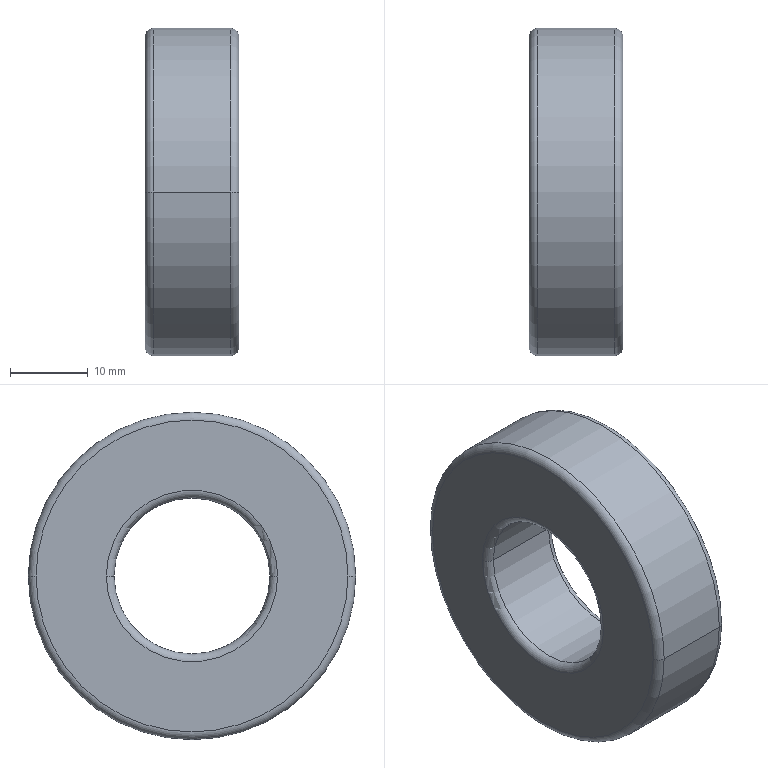Part | NX | features BREP 1 | 1 solid | 14 faces | box 12 x 42 x 42 mm | volume 12772 mm3 | torus 8 | cylinder 4 | plane 2 | commonest cylinder face diameters 20 x2 42 x2
STEP:
#1=CARTESIAN_POINT('',(12.,-20.,0.));
#2=VERTEX_POINT('',#1);
#3=CARTESIAN_POINT('',(12.,20.,0.));
#4=VERTEX_POINT('',#3);
#5=CARTESIAN_POINT('',(12.,0.,0.));
#6=DIRECTION('',(1.,0.,0.));
#7=DIRECTION('',(0.,-1.,0.));
#8=AXIS2_PLACEMENT_3D('',#5,#6,#7);
#9=CIRCLE('',#8,20.);
#10=EDGE_CURVE('',#2,#4,#9,.T.);
#11=ORIENTED_EDGE('',*,*,#10,.T.);
#12=CARTESIAN_POINT('',(12.,0.,0.));
#13=DIRECTION('',(1.,0.,0.));
#14=DIRECTION('',(0.,1.,0.));
#15=AXIS2_PLACEMENT_3D('',#12,#13,#14);
#16=CIRCLE('',#15,20.);
#17=EDGE_CURVE('',#4,#2,#16,.T.);
#18=ORIENTED_EDGE('',*,*,#17,.T.);
#19=EDGE_LOOP('',(#11,#18));
#20=FACE_BOUND('',#19,.T.);
#21=CARTESIAN_POINT('',(12.,-11.,0.));
#22=VERTEX_POINT('',#21);
#23=CARTESIAN_POINT('',(12.,11.,0.));
#24=VERTEX_POINT('',#23);
#25=CARTESIAN_POINT('',(12.,0.,0.));
#26=DIRECTION('',(-1.,0.,0.));
#27=DIRECTION('',(0.,-1.,0.));
#28=AXIS2_PLACEMENT_3D('',#25,#26,#27);
#29=CIRCLE('',#28,11.);
#30=EDGE_CURVE('',#22,#24,#29,.T.);
#31=ORIENTED_EDGE('',*,*,#30,.T.);
#32=CARTESIAN_POINT('',(12.,0.,0.));
#33=DIRECTION('',(-1.,0.,0.));
#34=DIRECTION('',(0.,1.,0.));
#35=AXIS2_PLACEMENT_3D('',#32,#33,#34);
#36=CIRCLE('',#35,11.);
#37=EDGE_CURVE('',#24,#22,#36,.T.);
#38=ORIENTED_EDGE('',*,*,#37,.T.);
#39=EDGE_LOOP('',(#31,#38));
#40=FACE_BOUND('',#39,.T.);
#41=CARTESIAN_POINT('',(12.,0.,0.));
#42=DIRECTION('',(1.,0.,0.));
#43=DIRECTION('',(0.,1.,0.));
#44=AXIS2_PLACEMENT_3D('',#41,#42,#43);
#45=PLANE('',#44);
#46=ADVANCED_FACE('',(#20,#40),#45,.T.);
#47=CARTESIAN_POINT('',(11.,21.,0.));
#48=VERTEX_POINT('',#47);
#49=CARTESIAN_POINT('',(11.,-21.,0.));
#50=VERTEX_POINT('',#49);
#51=CARTESIAN_POINT('',(11.,0.,0.));
#52=DIRECTION('',(1.,0.,0.));
#53=DIRECTION('',(0.,1.,0.));
#54=AXIS2_PLACEMENT_3D('',#51,#52,#53);
#55=CIRCLE('',#54,21.);
#56=EDGE_CURVE('',#48,#50,#55,.T.);
#57=ORIENTED_EDGE('',*,*,#56,.T.);
#58=CARTESIAN_POINT('',(11.,-20.,0.));
#59=DIRECTION('',(0.,0.,1.));
#60=DIRECTION('',(0.,-1.,0.));
#61=AXIS2_PLACEMENT_3D('',#58,#59,#60);
#62=CIRCLE('',#61,1.);
#63=EDGE_CURVE('',#50,#2,#62,.T.);
#64=ORIENTED_EDGE('',*,*,#63,.T.);
#65=ORIENTED_EDGE('',*,*,#17,.F.);
#66=CARTESIAN_POINT('',(11.,20.,0.));
#67=DIRECTION('',(0.,0.,-1.));
#68=DIRECTION('',(0.,1.,0.));
#69=AXIS2_PLACEMENT_3D('',#66,#67,#68);
#70=CIRCLE('',#69,1.);
#71=EDGE_CURVE('',#48,#4,#70,.T.);
#72=ORIENTED_EDGE('',*,*,#71,.F.);
#73=EDGE_LOOP('',(#57,#64,#65,#72));
#74=FACE_BOUND('',#73,.T.);
#75=CARTESIAN_POINT('',(11.,0.,0.));
#76=DIRECTION('',(1.,0.,0.));
#77=DIRECTION('',(0.,1.,0.));
#78=AXIS2_PLACEMENT_3D('',#75,#76,#77);
#79=TOROIDAL_SURFACE('',#78,20.,1.);
#80=ADVANCED_FACE('',(#74),#79,.T.);
#81=CARTESIAN_POINT('',(11.,0.,0.));
#82=DIRECTION('',(1.,0.,0.));
#83=DIRECTION('',(0.,-1.,0.));
#84=AXIS2_PLACEMENT_3D('',#81,#82,#83);
#85=CIRCLE('',#84,21.);
#86=EDGE_CURVE('',#50,#48,#85,.T.);
#87=ORIENTED_EDGE('',*,*,#86,.T.);
#88=ORIENTED_EDGE('',*,*,#71,.T.);
#89=ORIENTED_EDGE('',*,*,#10,.F.);
#90=ORIENTED_EDGE('',*,*,#63,.F.);
#91=EDGE_LOOP('',(#87,#88,#89,#90));
#92=FACE_BOUND('',#91,.T.);
#93=CARTESIAN_POINT('',(11.,0.,0.));
#94=DIRECTION('',(1.,0.,0.));
#95=DIRECTION('',(0.,-1.,0.));
#96=AXIS2_PLACEMENT_3D('',#93,#94,#95);
#97=TOROIDAL_SURFACE('',#96,20.,1.);
#98=ADVANCED_FACE('',(#92),#97,.T.);
#99=ORIENTED_EDGE('',*,*,#86,.F.);
#100=CARTESIAN_POINT('',(1.,-21.,0.));
#101=VERTEX_POINT('',#100);
#102=CARTESIAN_POINT('',(11.,-21.,0.));
#103=DIRECTION('',(-1.,0.,0.));
#104=VECTOR('',#103,1000.);
#105=LINE('',#102,#104);
#106=EDGE_CURVE('',#50,#101,#105,.T.);
#107=ORIENTED_EDGE('',*,*,#106,.T.);
#108=CARTESIAN_POINT('',(1.,21.,0.));
#109=VERTEX_POINT('',#108);
#110=CARTESIAN_POINT('',(1.,0.,0.));
#111=DIRECTION('',(-1.,0.,0.));
#112=DIRECTION('',(0.,1.,0.));
#113=AXIS2_PLACEMENT_3D('',#110,#111,#112);
#114=CIRCLE('',#113,21.);
#115=EDGE_CURVE('',#109,#101,#114,.T.);
#116=ORIENTED_EDGE('',*,*,#115,.F.);
#117=CARTESIAN_POINT('',(11.,21.,0.));
#118=DIRECTION('',(-1.,0.,0.));
#119=VECTOR('',#118,1000.);
#120=LINE('',#117,#119);
#121=EDGE_CURVE('',#48,#109,#120,.T.);
#122=ORIENTED_EDGE('',*,*,#121,.F.);
#123=EDGE_LOOP('',(#99,#107,#116,#122));
#124=FACE_BOUND('',#123,.T.);
#125=CARTESIAN_POINT('',(6.,0.,0.));
#126=DIRECTION('',(1.,0.,0.));
#127=DIRECTION('',(0.,1.,0.));
#128=AXIS2_PLACEMENT_3D('',#125,#126,#127);
#129=CYLINDRICAL_SURFACE('',#128,21.);
#130=ADVANCED_FACE('',(#124),#129,.T.);
#131=ORIENTED_EDGE('',*,*,#56,.F.);
#132=ORIENTED_EDGE('',*,*,#121,.T.);
#133=CARTESIAN_POINT('',(1.,0.,0.));
#134=DIRECTION('',(-1.,0.,0.));
#135=DIRECTION('',(0.,-1.,0.));
#136=AXIS2_PLACEMENT_3D('',#133,#134,#135);
#137=CIRCLE('',#136,21.);
#138=EDGE_CURVE('',#101,#109,#137,.T.);
#139=ORIENTED_EDGE('',*,*,#138,.F.);
#140=ORIENTED_EDGE('',*,*,#106,.F.);
#141=EDGE_LOOP('',(#131,#132,#139,#140));
#142=FACE_BOUND('',#141,.T.);
#143=CARTESIAN_POINT('',(6.,0.,0.));
#144=DIRECTION('',(1.,0.,0.));
#145=DIRECTION('',(0.,1.,0.));
#146=AXIS2_PLACEMENT_3D('',#143,#144,#145);
#147=CYLINDRICAL_SURFACE('',#146,21.);
#148=ADVANCED_FACE('',(#142),#147,.T.);
#149=CARTESIAN_POINT('',(0.,-20.,0.));
#150=VERTEX_POINT('',#149);
#151=CARTESIAN_POINT('',(0.,20.,0.));
#152=VERTEX_POINT('',#151);
#153=CARTESIAN_POINT('',(0.,0.,0.));
#154=DIRECTION('',(-1.,0.,0.));
#155=DIRECTION('',(0.,-1.,0.));
#156=AXIS2_PLACEMENT_3D('',#153,#154,#155);
#157=CIRCLE('',#156,20.);
#158=EDGE_CURVE('',#150,#152,#157,.T.);
#159=ORIENTED_EDGE('',*,*,#158,.F.);
#160=CARTESIAN_POINT('',(1.,-20.,0.));
#161=DIRECTION('',(0.,0.,1.));
#162=DIRECTION('',(-1.,0.,0.));
#163=AXIS2_PLACEMENT_3D('',#160,#161,#162);
#164=CIRCLE('',#163,1.);
#165=EDGE_CURVE('',#150,#101,#164,.T.);
#166=ORIENTED_EDGE('',*,*,#165,.T.);
#167=ORIENTED_EDGE('',*,*,#138,.T.);
#168=CARTESIAN_POINT('',(1.,20.,0.));
#169=DIRECTION('',(0.,0.,-1.));
#170=DIRECTION('',(-1.,0.,0.));
#171=AXIS2_PLACEMENT_3D('',#168,#169,#170);
#172=CIRCLE('',#171,1.);
#173=EDGE_CURVE('',#152,#109,#172,.T.);
#174=ORIENTED_EDGE('',*,*,#173,.F.);
#175=EDGE_LOOP('',(#159,#166,#167,#174));
#176=FACE_BOUND('',#175,.T.);
#177=CARTESIAN_POINT('',(1.,0.,0.));
#178=DIRECTION('',(1.,0.,0.));
#179=DIRECTION('',(0.,1.,0.));
#180=AXIS2_PLACEMENT_3D('',#177,#178,#179);
#181=TOROIDAL_SURFACE('',#180,20.,1.);
#182=ADVANCED_FACE('',(#176),#181,.T.);
#183=CARTESIAN_POINT('',(0.,0.,0.));
#184=DIRECTION('',(-1.,0.,0.));
#185=DIRECTION('',(0.,1.,0.));
#186=AXIS2_PLACEMENT_3D('',#183,#184,#185);
#187=CIRCLE('',#186,20.);
#188=EDGE_CURVE('',#152,#150,#187,.T.);
#189=ORIENTED_EDGE('',*,*,#188,.F.);
#190=ORIENTED_EDGE('',*,*,#173,.T.);
#191=ORIENTED_EDGE('',*,*,#115,.T.);
#192=ORIENTED_EDGE('',*,*,#165,.F.);
#193=EDGE_LOOP('',(#189,#190,#191,#192));
#194=FACE_BOUND('',#193,.T.);
#195=CARTESIAN_POINT('',(1.,0.,0.));
#196=DIRECTION('',(1.,0.,0.));
#197=DIRECTION('',(0.,-1.,0.));
#198=AXIS2_PLACEMENT_3D('',#195,#196,#197);
#199=TOROIDAL_SURFACE('',#198,20.,1.);
#200=ADVANCED_FACE('',(#194),#199,.T.);
#201=ORIENTED_EDGE('',*,*,#158,.T.);
#202=ORIENTED_EDGE('',*,*,#188,.T.);
#203=EDGE_LOOP('',(#201,#202));
#204=FACE_BOUND('',#203,.T.);
#205=CARTESIAN_POINT('',(0.,-11.,0.));
#206=VERTEX_POINT('',#205);
#207=CARTESIAN_POINT('',(0.,11.,0.));
#208=VERTEX_POINT('',#207);
#209=CARTESIAN_POINT('',(0.,0.,0.));
#210=DIRECTION('',(1.,0.,0.));
#211=DIRECTION('',(0.,-1.,0.));
#212=AXIS2_PLACEMENT_3D('',#209,#210,#211);
#213=CIRCLE('',#212,11.);
#214=EDGE_CURVE('',#206,#208,#213,.T.);
#215=ORIENTED_EDGE('',*,*,#214,.T.);
#216=CARTESIAN_POINT('',(0.,0.,0.));
#217=DIRECTION('',(1.,0.,0.));
#218=DIRECTION('',(0.,1.,0.));
#219=AXIS2_PLACEMENT_3D('',#216,#217,#218);
#220=CIRCLE('',#219,11.);
#221=EDGE_CURVE('',#208,#206,#220,.T.);
#222=ORIENTED_EDGE('',*,*,#221,.T.);
#223=EDGE_LOOP('',(#215,#222));
#224=FACE_BOUND('',#223,.T.);
#225=CARTESIAN_POINT('',(0.,0.,0.));
#226=DIRECTION('',(1.,0.,0.));
#227=DIRECTION('',(0.,1.,0.));
#228=AXIS2_PLACEMENT_3D('',#225,#226,#227);
#229=PLANE('',#228);
#230=ADVANCED_FACE('',(#204,#224),#229,.F.);
#231=CARTESIAN_POINT('',(1.,10.,0.));
#232=VERTEX_POINT('',#231);
#233=CARTESIAN_POINT('',(1.,-10.,0.));
#234=VERTEX_POINT('',#233);
#235=CARTESIAN_POINT('',(1.,0.,0.));
#236=DIRECTION('',(1.,0.,0.));
#237=DIRECTION('',(0.,1.,0.));
#238=AXIS2_PLACEMENT_3D('',#235,#236,#237);
#239=CIRCLE('',#238,10.);
#240=EDGE_CURVE('',#232,#234,#239,.T.);
#241=ORIENTED_EDGE('',*,*,#240,.T.);
#242=CARTESIAN_POINT('',(1.,-11.,0.));
#243=DIRECTION('',(0.,0.,1.));
#244=DIRECTION('',(0.,1.,0.));
#245=AXIS2_PLACEMENT_3D('',#242,#243,#244);
#246=CIRCLE('',#245,1.);
#247=EDGE_CURVE('',#234,#206,#246,.T.);
#248=ORIENTED_EDGE('',*,*,#247,.T.);
#249=ORIENTED_EDGE('',*,*,#221,.F.);
#250=CARTESIAN_POINT('',(1.,11.,0.));
#251=DIRECTION('',(0.,0.,-1.));
#252=DIRECTION('',(0.,-1.,0.));
#253=AXIS2_PLACEMENT_3D('',#250,#251,#252);
#254=CIRCLE('',#253,1.);
#255=EDGE_CURVE('',#232,#208,#254,.T.);
#256=ORIENTED_EDGE('',*,*,#255,.F.);
#257=EDGE_LOOP('',(#241,#248,#249,#256));
#258=FACE_BOUND('',#257,.T.);
#259=CARTESIAN_POINT('',(1.,0.,0.));
#260=DIRECTION('',(1.,0.,0.));
#261=DIRECTION('',(0.,1.,0.));
#262=AXIS2_PLACEMENT_3D('',#259,#260,#261);
#263=TOROIDAL_SURFACE('',#262,11.,1.);
#264=ADVANCED_FACE('',(#258),#263,.T.);
#265=CARTESIAN_POINT('',(1.,0.,0.));
#266=DIRECTION('',(1.,0.,0.));
#267=DIRECTION('',(0.,-1.,0.));
#268=AXIS2_PLACEMENT_3D('',#265,#266,#267);
#269=CIRCLE('',#268,10.);
#270=EDGE_CURVE('',#234,#232,#269,.T.);
#271=ORIENTED_EDGE('',*,*,#270,.T.);
#272=ORIENTED_EDGE('',*,*,#255,.T.);
#273=ORIENTED_EDGE('',*,*,#214,.F.);
#274=ORIENTED_EDGE('',*,*,#247,.F.);
#275=EDGE_LOOP('',(#271,#272,#273,#274));
#276=FACE_BOUND('',#275,.T.);
#277=CARTESIAN_POINT('',(1.,0.,0.));
#278=DIRECTION('',(1.,0.,0.));
#279=DIRECTION('',(0.,-1.,0.));
#280=AXIS2_PLACEMENT_3D('',#277,#278,#279);
#281=TOROIDAL_SURFACE('',#280,11.,1.);
#282=ADVANCED_FACE('',(#276),#281,.T.);
#283=CARTESIAN_POINT('',(11.,-10.,0.));
#284=VERTEX_POINT('',#283);
#285=CARTESIAN_POINT('',(11.,-10.,0.));
#286=DIRECTION('',(-1.,0.,0.));
#287=VECTOR('',#286,1000.);
#288=LINE('',#285,#287);
#289=EDGE_CURVE('',#284,#234,#288,.T.);
#290=ORIENTED_EDGE('',*,*,#289,.F.);
#291=CARTESIAN_POINT('',(11.,10.,0.));
#292=VERTEX_POINT('',#291);
#293=CARTESIAN_POINT('',(11.,0.,0.));
#294=DIRECTION('',(-1.,0.,0.));
#295=DIRECTION('',(0.,1.,0.));
#296=AXIS2_PLACEMENT_3D('',#293,#294,#295);
#297=CIRCLE('',#296,10.);
#298=EDGE_CURVE('',#292,#284,#297,.T.);
#299=ORIENTED_EDGE('',*,*,#298,.F.);
#300=CARTESIAN_POINT('',(11.,10.,0.));
#301=DIRECTION('',(-1.,0.,0.));
#302=VECTOR('',#301,1000.);
#303=LINE('',#300,#302);
#304=EDGE_CURVE('',#292,#232,#303,.T.);
#305=ORIENTED_EDGE('',*,*,#304,.T.);
#306=ORIENTED_EDGE('',*,*,#270,.F.);
#307=EDGE_LOOP('',(#290,#299,#305,#306));
#308=FACE_BOUND('',#307,.T.);
#309=CARTESIAN_POINT('',(6.,0.,0.));
#310=DIRECTION('',(1.,0.,0.));
#311=DIRECTION('',(0.,1.,0.));
#312=AXIS2_PLACEMENT_3D('',#309,#310,#311);
#313=CYLINDRICAL_SURFACE('',#312,10.);
#314=ADVANCED_FACE('',(#308),#313,.F.);
#315=ORIENTED_EDGE('',*,*,#304,.F.);
#316=CARTESIAN_POINT('',(11.,0.,0.));
#317=DIRECTION('',(-1.,0.,0.));
#318=DIRECTION('',(0.,-1.,0.));
#319=AXIS2_PLACEMENT_3D('',#316,#317,#318);
#320=CIRCLE('',#319,10.);
#321=EDGE_CURVE('',#284,#292,#320,.T.);
#322=ORIENTED_EDGE('',*,*,#321,.F.);
#323=ORIENTED_EDGE('',*,*,#289,.T.);
#324=ORIENTED_EDGE('',*,*,#240,.F.);
#325=EDGE_LOOP('',(#315,#322,#323,#324));
#326=FACE_BOUND('',#325,.T.);
#327=CARTESIAN_POINT('',(6.,0.,0.));
#328=DIRECTION('',(1.,0.,0.));
#329=DIRECTION('',(0.,1.,0.));
#330=AXIS2_PLACEMENT_3D('',#327,#328,#329);
#331=CYLINDRICAL_SURFACE('',#330,10.);
#332=ADVANCED_FACE('',(#326),#331,.F.);
#333=ORIENTED_EDGE('',*,*,#30,.F.);
#334=CARTESIAN_POINT('',(11.,-11.,0.));
#335=DIRECTION('',(0.,0.,1.));
#336=DIRECTION('',(1.,0.,0.));
#337=AXIS2_PLACEMENT_3D('',#334,#335,#336);
#338=CIRCLE('',#337,1.);
#339=EDGE_CURVE('',#22,#284,#338,.T.);
#340=ORIENTED_EDGE('',*,*,#339,.T.);
#341=ORIENTED_EDGE('',*,*,#321,.T.);
#342=CARTESIAN_POINT('',(11.,11.,0.));
#343=DIRECTION('',(0.,0.,-1.));
#344=DIRECTION('',(1.,0.,0.));
#345=AXIS2_PLACEMENT_3D('',#342,#343,#344);
#346=CIRCLE('',#345,1.);
#347=EDGE_CURVE('',#24,#292,#346,.T.);
#348=ORIENTED_EDGE('',*,*,#347,.F.);
#349=EDGE_LOOP('',(#333,#340,#341,#348));
#350=FACE_BOUND('',#349,.T.);
#351=CARTESIAN_POINT('',(11.,0.,0.));
#352=DIRECTION('',(1.,0.,0.));
#353=DIRECTION('',(0.,1.,0.));
#354=AXIS2_PLACEMENT_3D('',#351,#352,#353);
#355=TOROIDAL_SURFACE('',#354,11.,1.);
#356=ADVANCED_FACE('',(#350),#355,.T.);
#357=ORIENTED_EDGE('',*,*,#37,.F.);
#358=ORIENTED_EDGE('',*,*,#347,.T.);
#359=ORIENTED_EDGE('',*,*,#298,.T.);
#360=ORIENTED_EDGE('',*,*,#339,.F.);
#361=EDGE_LOOP('',(#357,#358,#359,#360));
#362=FACE_BOUND('',#361,.T.);
#363=CARTESIAN_POINT('',(11.,0.,0.));
#364=DIRECTION('',(1.,0.,0.));
#365=DIRECTION('',(0.,-1.,0.));
#366=AXIS2_PLACEMENT_3D('',#363,#364,#365);
#367=TOROIDAL_SURFACE('',#366,11.,1.);
#368=ADVANCED_FACE('',(#362),#367,.T.);
#369=CLOSED_SHELL('',(#46,#80,#98,#130,#148,#182,#200,#230,#264,#282,#314,#332,#356,#368));
#370=MANIFOLD_SOLID_BREP('',#369);
#371=(LENGTH_UNIT()NAMED_UNIT(*)SI_UNIT(.MILLI.,.METRE.));
#372=UNCERTAINTY_MEASURE_WITH_UNIT(LENGTH_MEASURE(0.00001),#371,'','');
#373=(NAMED_UNIT(*)PLANE_ANGLE_UNIT()SI_UNIT($,.RADIAN.));
#374=(NAMED_UNIT(*)SI_UNIT($,.STERADIAN.)SOLID_ANGLE_UNIT());
#375=(GEOMETRIC_REPRESENTATION_CONTEXT(3)GLOBAL_UNCERTAINTY_ASSIGNED_CONTEXT((#372))GLOBAL_UNIT_ASSIGNED_CONTEXT((#371,#373,#374))REPRESENTATION_CONTEXT('',''));
#376=ADVANCED_BREP_SHAPE_REPRESENTATION('',(#370),#375);